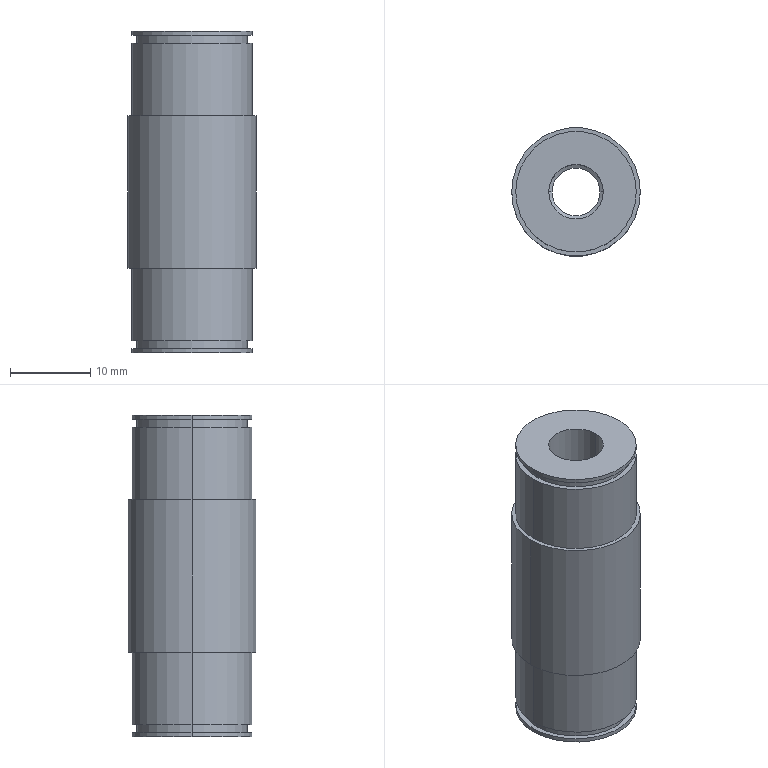Part | STEP file | Driven shaft | 1 solid | 30 faces | box 16 x 16 x 40 mm | volume 6026 mm3 | cylinder 18 | plane 8 | cone 4 | commonest cylinder face diameters 15 x8 6.8 x4 13.8 x4 16 x2